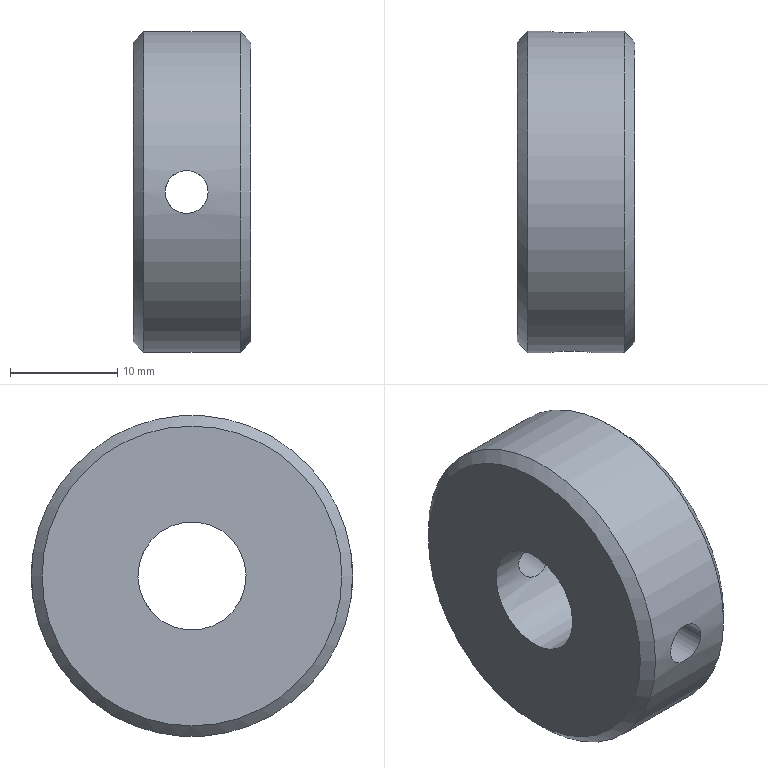Part | STEP file | SN10_001_012_TRAVA | 1 solid | 8 faces | box 11 x 30 x 30 mm | volume 6549 mm3 | cylinder 4 | plane 2 | cone 2 | commonest cylinder face diameters 4 x2 10.106 x1 30 x1